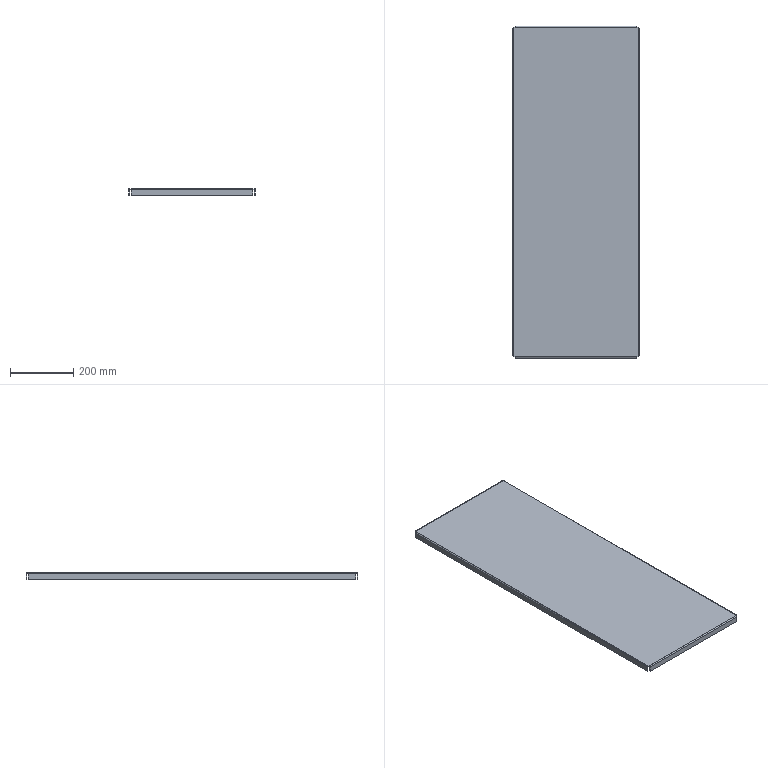Part | SolidWorks | features BaseBody 1 | 1 solid | 50 faces | box 398 x 1046 x 20 mm | volume 1158388 mm3 | plane 42 | cylinder 8 | commonest cylinder face diameters 1.473 x4 6.473 x4
STEP:
#1=CARTESIAN_POINT('',(-192.,-520.5,-20.));
#2=VERTEX_POINT('',#1);
#3=CARTESIAN_POINT('',(192.,-520.5,-20.));
#4=VERTEX_POINT('',#3);
#5=CARTESIAN_POINT('',(192.,-520.5,-20.));
#6=DIRECTION('',(1.,0.,0.));
#7=VECTOR('',#6,1000.);
#8=LINE('',#5,#7);
#9=EDGE_CURVE('',#2,#4,#8,.T.);
#10=ORIENTED_EDGE('',*,*,#9,.T.);
#11=CARTESIAN_POINT('',(192.,-523.,-20.));
#12=VERTEX_POINT('',#11);
#13=CARTESIAN_POINT('',(192.,-523.,-20.));
#14=DIRECTION('',(0.,1.,0.));
#15=VECTOR('',#14,1000.);
#16=LINE('',#13,#15);
#17=EDGE_CURVE('',#12,#4,#16,.T.);
#18=ORIENTED_EDGE('',*,*,#17,.F.);
#19=CARTESIAN_POINT('',(-192.,-523.,-20.));
#20=VERTEX_POINT('',#19);
#21=CARTESIAN_POINT('',(0.,-523.,-20.));
#22=DIRECTION('',(1.,0.,0.));
#23=VECTOR('',#22,1000.);
#24=LINE('',#21,#23);
#25=EDGE_CURVE('',#20,#12,#24,.T.);
#26=ORIENTED_EDGE('',*,*,#25,.F.);
#27=CARTESIAN_POINT('',(-192.,-523.,-20.));
#28=DIRECTION('',(0.,1.,0.));
#29=VECTOR('',#28,1000.);
#30=LINE('',#27,#29);
#31=EDGE_CURVE('',#20,#2,#30,.T.);
#32=ORIENTED_EDGE('',*,*,#31,.T.);
#33=EDGE_LOOP('',(#10,#18,#26,#32));
#34=FACE_OUTER_BOUND('',#33,.T.);
#35=CARTESIAN_POINT('',(192.,-523.,-20.));
#36=DIRECTION('',(0.,0.,1.));
#37=DIRECTION('',(0.,-1.,0.));
#38=AXIS2_PLACEMENT_3D('',#35,#36,#37);
#39=PLANE('',#38);
#40=ADVANCED_FACE('',(#34),#39,.F.);
#41=CARTESIAN_POINT('',(-192.,-520.5,-3.237));
#42=VERTEX_POINT('',#41);
#43=CARTESIAN_POINT('',(-192.,-520.5,-20.));
#44=DIRECTION('',(0.,0.,-1.));
#45=VECTOR('',#44,1000.);
#46=LINE('',#43,#45);
#47=EDGE_CURVE('',#42,#2,#46,.T.);
#48=ORIENTED_EDGE('',*,*,#47,.F.);
#49=CARTESIAN_POINT('',(192.,-520.5,-3.237));
#50=VERTEX_POINT('',#49);
#51=CARTESIAN_POINT('',(192.,-520.5,-3.237));
#52=DIRECTION('',(-1.,0.,0.));
#53=VECTOR('',#52,1000.);
#54=LINE('',#51,#53);
#55=EDGE_CURVE('',#50,#42,#54,.T.);
#56=ORIENTED_EDGE('',*,*,#55,.F.);
#57=CARTESIAN_POINT('',(192.,-520.5,-2.5));
#58=DIRECTION('',(0.,0.,1.));
#59=VECTOR('',#58,1000.);
#60=LINE('',#57,#59);
#61=EDGE_CURVE('',#4,#50,#60,.T.);
#62=ORIENTED_EDGE('',*,*,#61,.F.);
#63=ORIENTED_EDGE('',*,*,#9,.F.);
#64=EDGE_LOOP('',(#48,#56,#62,#63));
#65=FACE_OUTER_BOUND('',#64,.T.);
#66=CARTESIAN_POINT('',(0.,-520.5,0.));
#67=DIRECTION('',(0.,1.,0.));
#68=DIRECTION('',(1.,0.,0.));
#69=AXIS2_PLACEMENT_3D('',#66,#67,#68);
#70=PLANE('',#69);
#71=ADVANCED_FACE('',(#65),#70,.T.);
#72=CARTESIAN_POINT('',(-192.,-523.,-3.237));
#73=VERTEX_POINT('',#72);
#74=CARTESIAN_POINT('',(192.,-523.,-3.237));
#75=VERTEX_POINT('',#74);
#76=CARTESIAN_POINT('',(192.,-523.,-3.237));
#77=DIRECTION('',(1.,0.,0.));
#78=VECTOR('',#77,1000.);
#79=LINE('',#76,#78);
#80=EDGE_CURVE('',#73,#75,#79,.T.);
#81=ORIENTED_EDGE('',*,*,#80,.F.);
#82=CARTESIAN_POINT('',(-192.,-523.,0.));
#83=DIRECTION('',(0.,0.,-1.));
#84=VECTOR('',#83,1000.);
#85=LINE('',#82,#84);
#86=EDGE_CURVE('',#73,#20,#85,.T.);
#87=ORIENTED_EDGE('',*,*,#86,.T.);
#88=ORIENTED_EDGE('',*,*,#25,.T.);
#89=CARTESIAN_POINT('',(192.,-523.,0.));
#90=DIRECTION('',(0.,0.,1.));
#91=VECTOR('',#90,1000.);
#92=LINE('',#89,#91);
#93=EDGE_CURVE('',#12,#75,#92,.T.);
#94=ORIENTED_EDGE('',*,*,#93,.T.);
#95=EDGE_LOOP('',(#81,#87,#88,#94));
#96=FACE_OUTER_BOUND('',#95,.T.);
#97=CARTESIAN_POINT('',(0.,-523.,0.));
#98=DIRECTION('',(0.,1.,0.));
#99=DIRECTION('',(1.,0.,0.));
#100=AXIS2_PLACEMENT_3D('',#97,#98,#99);
#101=PLANE('',#100);
#102=ADVANCED_FACE('',(#96),#101,.F.);
#103=CARTESIAN_POINT('',(192.,-523.,-3.237));
#104=DIRECTION('',(0.,-1.,0.));
#105=VECTOR('',#104,1000.);
#106=LINE('',#103,#105);
#107=EDGE_CURVE('',#50,#75,#106,.T.);
#108=ORIENTED_EDGE('',*,*,#107,.T.);
#109=ORIENTED_EDGE('',*,*,#93,.F.);
#110=ORIENTED_EDGE('',*,*,#17,.T.);
#111=ORIENTED_EDGE('',*,*,#61,.T.);
#112=EDGE_LOOP('',(#108,#109,#110,#111));
#113=FACE_OUTER_BOUND('',#112,.T.);
#114=CARTESIAN_POINT('',(192.,-523.,-2.5));
#115=DIRECTION('',(-1.,0.,0.));
#116=DIRECTION('',(0.,1.,0.));
#117=AXIS2_PLACEMENT_3D('',#114,#115,#116);
#118=PLANE('',#117);
#119=ADVANCED_FACE('',(#113),#118,.F.);
#120=CARTESIAN_POINT('',(-192.,-520.5,-3.237));
#121=DIRECTION('',(0.,-1.,0.));
#122=VECTOR('',#121,1000.);
#123=LINE('',#120,#122);
#124=EDGE_CURVE('',#42,#73,#123,.T.);
#125=ORIENTED_EDGE('',*,*,#124,.F.);
#126=ORIENTED_EDGE('',*,*,#47,.T.);
#127=ORIENTED_EDGE('',*,*,#31,.F.);
#128=ORIENTED_EDGE('',*,*,#86,.F.);
#129=EDGE_LOOP('',(#125,#126,#127,#128));
#130=FACE_OUTER_BOUND('',#129,.T.);
#131=CARTESIAN_POINT('',(-192.,-523.,-20.));
#132=DIRECTION('',(1.,0.,0.));
#133=DIRECTION('',(0.,1.,0.));
#134=AXIS2_PLACEMENT_3D('',#131,#132,#133);
#135=PLANE('',#134);
#136=ADVANCED_FACE('',(#130),#135,.F.);
#137=CARTESIAN_POINT('',(-192.,-519.763,-2.5));
#138=VERTEX_POINT('',#137);
#139=CARTESIAN_POINT('',(192.,-519.763,-2.5));
#140=VERTEX_POINT('',#139);
#141=CARTESIAN_POINT('',(-192.,-519.763,-2.5));
#142=DIRECTION('',(1.,0.,0.));
#143=VECTOR('',#142,1000.);
#144=LINE('',#141,#143);
#145=EDGE_CURVE('',#138,#140,#144,.T.);
#146=ORIENTED_EDGE('',*,*,#145,.T.);
#147=CARTESIAN_POINT('',(192.,-519.763,-3.237));
#148=DIRECTION('',(1.,0.,0.));
#149=DIRECTION('',(0.,0.,1.));
#150=AXIS2_PLACEMENT_3D('',#147,#148,#149);
#151=CIRCLE('',#150,0.7366);
#152=EDGE_CURVE('',#140,#50,#151,.T.);
#153=ORIENTED_EDGE('',*,*,#152,.T.);
#154=ORIENTED_EDGE('',*,*,#55,.T.);
#155=CARTESIAN_POINT('',(-192.,-519.763,-3.237));
#156=DIRECTION('',(-1.,0.,0.));
#157=DIRECTION('',(0.,0.,1.));
#158=AXIS2_PLACEMENT_3D('',#155,#156,#157);
#159=CIRCLE('',#158,0.7366);
#160=EDGE_CURVE('',#42,#138,#159,.T.);
#161=ORIENTED_EDGE('',*,*,#160,.T.);
#162=EDGE_LOOP('',(#146,#153,#154,#161));
#163=FACE_OUTER_BOUND('',#162,.T.);
#164=CARTESIAN_POINT('',(-192.,-519.763,-3.237));
#165=DIRECTION('',(-1.,0.,0.));
#166=DIRECTION('',(0.,-1.,0.));
#167=AXIS2_PLACEMENT_3D('',#164,#165,#166);
#168=CYLINDRICAL_SURFACE('',#167,0.7366);
#169=ADVANCED_FACE('',(#163),#168,.F.);
#170=CARTESIAN_POINT('',(-192.,-519.763,0.));
#171=VERTEX_POINT('',#170);
#172=CARTESIAN_POINT('',(192.,-519.763,0.));
#173=VERTEX_POINT('',#172);
#174=CARTESIAN_POINT('',(-192.,-519.763,0.));
#175=DIRECTION('',(1.,0.,0.));
#176=VECTOR('',#175,1000.);
#177=LINE('',#174,#176);
#178=EDGE_CURVE('',#171,#173,#177,.T.);
#179=ORIENTED_EDGE('',*,*,#178,.F.);
#180=CARTESIAN_POINT('',(-192.,-522.915,-2.5));
#181=VERTEX_POINT('',#180);
#182=CARTESIAN_POINT('',(-192.,-519.763,-3.237));
#183=DIRECTION('',(-1.,0.,0.));
#184=DIRECTION('',(0.,0.,1.));
#185=AXIS2_PLACEMENT_3D('',#182,#183,#184);
#186=CIRCLE('',#185,3.237);
#187=EDGE_CURVE('',#181,#171,#186,.T.);
#188=ORIENTED_EDGE('',*,*,#187,.F.);
#189=CARTESIAN_POINT('',(-192.,-519.763,-3.237));
#190=DIRECTION('',(-1.,0.,0.));
#191=DIRECTION('',(0.,0.,1.));
#192=AXIS2_PLACEMENT_3D('',#189,#190,#191);
#193=CIRCLE('',#192,3.237);
#194=EDGE_CURVE('',#73,#181,#193,.T.);
#195=ORIENTED_EDGE('',*,*,#194,.F.);
#196=ORIENTED_EDGE('',*,*,#80,.T.);
#197=CARTESIAN_POINT('',(192.,-522.915,-2.5));
#198=VERTEX_POINT('',#197);
#199=CARTESIAN_POINT('',(192.,-519.763,-3.237));
#200=DIRECTION('',(1.,0.,0.));
#201=DIRECTION('',(0.,0.,1.));
#202=AXIS2_PLACEMENT_3D('',#199,#200,#201);
#203=CIRCLE('',#202,3.237);
#204=EDGE_CURVE('',#198,#75,#203,.T.);
#205=ORIENTED_EDGE('',*,*,#204,.F.);
#206=CARTESIAN_POINT('',(192.,-519.763,-3.237));
#207=DIRECTION('',(1.,0.,0.));
#208=DIRECTION('',(0.,0.,1.));
#209=AXIS2_PLACEMENT_3D('',#206,#207,#208);
#210=CIRCLE('',#209,3.237);
#211=EDGE_CURVE('',#173,#198,#210,.T.);
#212=ORIENTED_EDGE('',*,*,#211,.F.);
#213=EDGE_LOOP('',(#179,#188,#195,#196,#205,#212));
#214=FACE_OUTER_BOUND('',#213,.T.);
#215=CARTESIAN_POINT('',(-192.,-519.763,-3.237));
#216=DIRECTION('',(-1.,0.,0.));
#217=DIRECTION('',(0.,-1.,0.));
#218=AXIS2_PLACEMENT_3D('',#215,#216,#217);
#219=CYLINDRICAL_SURFACE('',#218,3.237);
#220=ADVANCED_FACE('',(#214),#219,.T.);
#221=ORIENTED_EDGE('',*,*,#194,.T.);
#222=CARTESIAN_POINT('',(-192.,-523.,-2.5));
#223=DIRECTION('',(0.,1.,0.));
#224=VECTOR('',#223,1000.);
#225=LINE('',#222,#224);
#226=EDGE_CURVE('',#181,#138,#225,.T.);
#227=ORIENTED_EDGE('',*,*,#226,.T.);
#228=ORIENTED_EDGE('',*,*,#160,.F.);
#229=ORIENTED_EDGE('',*,*,#124,.T.);
#230=EDGE_LOOP('',(#221,#227,#228,#229));
#231=FACE_OUTER_BOUND('',#230,.T.);
#232=CARTESIAN_POINT('',(-192.,-519.763,-3.237));
#233=DIRECTION('',(1.,0.,0.));
#234=DIRECTION('',(0.,1.,0.));
#235=AXIS2_PLACEMENT_3D('',#232,#233,#234);
#236=PLANE('',#235);
#237=ADVANCED_FACE('',(#231),#236,.F.);
#238=ORIENTED_EDGE('',*,*,#152,.F.);
#239=CARTESIAN_POINT('',(192.,-519.763,-2.5));
#240=DIRECTION('',(0.,-1.,0.));
#241=VECTOR('',#240,1000.);
#242=LINE('',#239,#241);
#243=EDGE_CURVE('',#140,#198,#242,.T.);
#244=ORIENTED_EDGE('',*,*,#243,.T.);
#245=ORIENTED_EDGE('',*,*,#204,.T.);
#246=ORIENTED_EDGE('',*,*,#107,.F.);
#247=EDGE_LOOP('',(#238,#244,#245,#246));
#248=FACE_OUTER_BOUND('',#247,.T.);
#249=CARTESIAN_POINT('',(192.,-519.763,-3.237));
#250=DIRECTION('',(1.,0.,0.));
#251=DIRECTION('',(0.,1.,0.));
#252=AXIS2_PLACEMENT_3D('',#249,#250,#251);
#253=PLANE('',#252);
#254=ADVANCED_FACE('',(#248),#253,.T.);
#255=CARTESIAN_POINT('',(196.5,-516.,-20.));
#256=VERTEX_POINT('',#255);
#257=CARTESIAN_POINT('',(196.5,516.,-20.));
#258=VERTEX_POINT('',#257);
#259=CARTESIAN_POINT('',(196.5,516.,-20.));
#260=DIRECTION('',(0.,1.,0.));
#261=VECTOR('',#260,1000.);
#262=LINE('',#259,#261);
#263=EDGE_CURVE('',#256,#258,#262,.T.);
#264=ORIENTED_EDGE('',*,*,#263,.T.);
#265=CARTESIAN_POINT('',(199.,516.,-20.));
#266=VERTEX_POINT('',#265);
#267=CARTESIAN_POINT('',(199.,516.,-20.));
#268=DIRECTION('',(-1.,0.,0.));
#269=VECTOR('',#268,1000.);
#270=LINE('',#267,#269);
#271=EDGE_CURVE('',#266,#258,#270,.T.);
#272=ORIENTED_EDGE('',*,*,#271,.F.);
#273=CARTESIAN_POINT('',(199.,-516.,-20.));
#274=VERTEX_POINT('',#273);
#275=CARTESIAN_POINT('',(199.,0.,-20.));
#276=DIRECTION('',(0.,1.,0.));
#277=VECTOR('',#276,1000.);
#278=LINE('',#275,#277);
#279=EDGE_CURVE('',#274,#266,#278,.T.);
#280=ORIENTED_EDGE('',*,*,#279,.F.);
#281=CARTESIAN_POINT('',(199.,-516.,-20.));
#282=DIRECTION('',(-1.,0.,0.));
#283=VECTOR('',#282,1000.);
#284=LINE('',#281,#283);
#285=EDGE_CURVE('',#274,#256,#284,.T.);
#286=ORIENTED_EDGE('',*,*,#285,.T.);
#287=EDGE_LOOP('',(#264,#272,#280,#286));
#288=FACE_OUTER_BOUND('',#287,.T.);
#289=CARTESIAN_POINT('',(199.,516.,-20.));
#290=DIRECTION('',(0.,0.,1.));
#291=DIRECTION('',(1.,0.,0.));
#292=AXIS2_PLACEMENT_3D('',#289,#290,#291);
#293=PLANE('',#292);
#294=ADVANCED_FACE('',(#288),#293,.F.);
#295=CARTESIAN_POINT('',(196.5,-516.,-3.237));
#296=VERTEX_POINT('',#295);
#297=CARTESIAN_POINT('',(196.5,-516.,-20.));
#298=DIRECTION('',(0.,0.,-1.));
#299=VECTOR('',#298,1000.);
#300=LINE('',#297,#299);
#301=EDGE_CURVE('',#296,#256,#300,.T.);
#302=ORIENTED_EDGE('',*,*,#301,.F.);
#303=CARTESIAN_POINT('',(196.5,516.,-3.237));
#304=VERTEX_POINT('',#303);
#305=CARTESIAN_POINT('',(196.5,516.,-3.237));
#306=DIRECTION('',(0.,-1.,0.));
#307=VECTOR('',#306,1000.);
#308=LINE('',#305,#307);
#309=EDGE_CURVE('',#304,#296,#308,.T.);
#310=ORIENTED_EDGE('',*,*,#309,.F.);
#311=CARTESIAN_POINT('',(196.5,516.,-2.5));
#312=DIRECTION('',(0.,0.,1.));
#313=VECTOR('',#312,1000.);
#314=LINE('',#311,#313);
#315=EDGE_CURVE('',#258,#304,#314,.T.);
#316=ORIENTED_EDGE('',*,*,#315,.F.);
#317=ORIENTED_EDGE('',*,*,#263,.F.);
#318=EDGE_LOOP('',(#302,#310,#316,#317));
#319=FACE_OUTER_BOUND('',#318,.T.);
#320=CARTESIAN_POINT('',(196.5,0.,0.));
#321=DIRECTION('',(-1.,0.,0.));
#322=DIRECTION('',(0.,0.,1.));
#323=AXIS2_PLACEMENT_3D('',#320,#321,#322);
#324=PLANE('',#323);
#325=ADVANCED_FACE('',(#319),#324,.T.);
#326=CARTESIAN_POINT('',(199.,-516.,-3.237));
#327=VERTEX_POINT('',#326);
#328=CARTESIAN_POINT('',(199.,516.,-3.237));
#329=VERTEX_POINT('',#328);
#330=CARTESIAN_POINT('',(199.,516.,-3.237));
#331=DIRECTION('',(0.,1.,0.));
#332=VECTOR('',#331,1000.);
#333=LINE('',#330,#332);
#334=EDGE_CURVE('',#327,#329,#333,.T.);
#335=ORIENTED_EDGE('',*,*,#334,.F.);
#336=CARTESIAN_POINT('',(199.,-516.,0.));
#337=DIRECTION('',(0.,0.,-1.));
#338=VECTOR('',#337,1000.);
#339=LINE('',#336,#338);
#340=EDGE_CURVE('',#327,#274,#339,.T.);
#341=ORIENTED_EDGE('',*,*,#340,.T.);
#342=ORIENTED_EDGE('',*,*,#279,.T.);
#343=CARTESIAN_POINT('',(199.,516.,0.));
#344=DIRECTION('',(0.,0.,1.));
#345=VECTOR('',#344,1000.);
#346=LINE('',#343,#345);
#347=EDGE_CURVE('',#266,#329,#346,.T.);
#348=ORIENTED_EDGE('',*,*,#347,.T.);
#349=EDGE_LOOP('',(#335,#341,#342,#348));
#350=FACE_OUTER_BOUND('',#349,.T.);
#351=CARTESIAN_POINT('',(199.,0.,0.));
#352=DIRECTION('',(-1.,0.,0.));
#353=DIRECTION('',(0.,0.,1.));
#354=AXIS2_PLACEMENT_3D('',#351,#352,#353);
#355=PLANE('',#354);
#356=ADVANCED_FACE('',(#350),#355,.F.);
#357=CARTESIAN_POINT('',(199.,516.,-3.237));
#358=DIRECTION('',(1.,0.,0.));
#359=VECTOR('',#358,1000.);
#360=LINE('',#357,#359);
#361=EDGE_CURVE('',#304,#329,#360,.T.);
#362=ORIENTED_EDGE('',*,*,#361,.T.);
#363=ORIENTED_EDGE('',*,*,#347,.F.);
#364=ORIENTED_EDGE('',*,*,#271,.T.);
#365=ORIENTED_EDGE('',*,*,#315,.T.);
#366=EDGE_LOOP('',(#362,#363,#364,#365));
#367=FACE_OUTER_BOUND('',#366,.T.);
#368=CARTESIAN_POINT('',(199.,516.,-2.5));
#369=DIRECTION('',(0.,-1.,0.));
#370=DIRECTION('',(0.,0.,-1.));
#371=AXIS2_PLACEMENT_3D('',#368,#369,#370);
#372=PLANE('',#371);
#373=ADVANCED_FACE('',(#367),#372,.F.);
#374=CARTESIAN_POINT('',(196.5,-516.,-3.237));
#375=DIRECTION('',(1.,0.,0.));
#376=VECTOR('',#375,1000.);
#377=LINE('',#374,#376);
#378=EDGE_CURVE('',#296,#327,#377,.T.);
#379=ORIENTED_EDGE('',*,*,#378,.F.);
#380=ORIENTED_EDGE('',*,*,#301,.T.);
#381=ORIENTED_EDGE('',*,*,#285,.F.);
#382=ORIENTED_EDGE('',*,*,#340,.F.);
#383=EDGE_LOOP('',(#379,#380,#381,#382));
#384=FACE_OUTER_BOUND('',#383,.T.);
#385=CARTESIAN_POINT('',(199.,-516.,-20.));
#386=DIRECTION('',(0.,1.,0.));
#387=DIRECTION('',(0.,0.,-1.));
#388=AXIS2_PLACEMENT_3D('',#385,#386,#387);
#389=PLANE('',#388);
#390=ADVANCED_FACE('',(#384),#389,.F.);
#391=CARTESIAN_POINT('',(195.763,-516.,-2.5));
#392=VERTEX_POINT('',#391);
#393=CARTESIAN_POINT('',(195.763,516.,-2.5));
#394=VERTEX_POINT('',#393);
#395=CARTESIAN_POINT('',(195.763,-516.,-2.5));
#396=DIRECTION('',(0.,1.,0.));
#397=VECTOR('',#396,1000.);
#398=LINE('',#395,#397);
#399=EDGE_CURVE('',#392,#394,#398,.T.);
#400=ORIENTED_EDGE('',*,*,#399,.T.);
#401=CARTESIAN_POINT('',(195.763,516.,-3.237));
#402=DIRECTION('',(0.,1.,0.));
#403=DIRECTION('',(0.,0.,-1.));
#404=AXIS2_PLACEMENT_3D('',#401,#402,#403);
#405=CIRCLE('',#404,0.7366);
#406=EDGE_CURVE('',#394,#304,#405,.T.);
#407=ORIENTED_EDGE('',*,*,#406,.T.);
#408=ORIENTED_EDGE('',*,*,#309,.T.);
#409=CARTESIAN_POINT('',(195.763,-516.,-3.237));
#410=DIRECTION('',(0.,-1.,0.));
#411=DIRECTION('',(0.,0.,-1.));
#412=AXIS2_PLACEMENT_3D('',#409,#410,#411);
#413=CIRCLE('',#412,0.7366);
#414=EDGE_CURVE('',#296,#392,#413,.T.);
#415=ORIENTED_EDGE('',*,*,#414,.T.);
#416=EDGE_LOOP('',(#400,#407,#408,#415));
#417=FACE_OUTER_BOUND('',#416,.T.);
#418=CARTESIAN_POINT('',(195.763,-516.,-3.237));
#419=DIRECTION('',(0.,-1.,0.));
#420=DIRECTION('',(1.,0.,0.));
#421=AXIS2_PLACEMENT_3D('',#418,#419,#420);
#422=CYLINDRICAL_SURFACE('',#421,0.7366);
#423=ADVANCED_FACE('',(#417),#422,.F.);
#424=CARTESIAN_POINT('',(195.763,-516.,0.));
#425=VERTEX_POINT('',#424);
#426=CARTESIAN_POINT('',(195.763,516.,0.));
#427=VERTEX_POINT('',#426);
#428=CARTESIAN_POINT('',(195.763,-516.,0.));
#429=DIRECTION('',(0.,1.,0.));
#430=VECTOR('',#429,1000.);
#431=LINE('',#428,#430);
#432=EDGE_CURVE('',#425,#427,#431,.T.);
#433=ORIENTED_EDGE('',*,*,#432,.F.);
#434=CARTESIAN_POINT('',(198.915,-516.,-2.5));
#435=VERTEX_POINT('',#434);
#436=CARTESIAN_POINT('',(195.763,-516.,-3.237));
#437=DIRECTION('',(0.,-1.,0.));
#438=DIRECTION('',(0.,0.,-1.));
#439=AXIS2_PLACEMENT_3D('',#436,#437,#438);
#440=CIRCLE('',#439,3.237);
#441=EDGE_CURVE('',#435,#425,#440,.T.);
#442=ORIENTED_EDGE('',*,*,#441,.F.);
#443=CARTESIAN_POINT('',(195.763,-516.,-3.237));
#444=DIRECTION('',(0.,-1.,0.));
#445=DIRECTION('',(0.,0.,-1.));
#446=AXIS2_PLACEMENT_3D('',#443,#444,#445);
#447=CIRCLE('',#446,3.237);
#448=EDGE_CURVE('',#327,#435,#447,.T.);
#449=ORIENTED_EDGE('',*,*,#448,.F.);
#450=ORIENTED_EDGE('',*,*,#334,.T.);
#451=CARTESIAN_POINT('',(198.915,516.,-2.5));
#452=VERTEX_POINT('',#451);
#453=CARTESIAN_POINT('',(195.763,516.,-3.237));
#454=DIRECTION('',(0.,1.,0.));
#455=DIRECTION('',(0.,0.,-1.));
#456=AXIS2_PLACEMENT_3D('',#453,#454,#455);
#457=CIRCLE('',#456,3.237);
#458=EDGE_CURVE('',#452,#329,#457,.T.);
#459=ORIENTED_EDGE('',*,*,#458,.F.);
#460=CARTESIAN_POINT('',(195.763,516.,-3.237));
#461=DIRECTION('',(0.,1.,0.));
#462=DIRECTION('',(0.,0.,-1.));
#463=AXIS2_PLACEMENT_3D('',#460,#461,#462);
#464=CIRCLE('',#463,3.237);
#465=EDGE_CURVE('',#427,#452,#464,.T.);
#466=ORIENTED_EDGE('',*,*,#465,.F.);
#467=EDGE_LOOP('',(#433,#442,#449,#450,#459,#466));
#468=FACE_OUTER_BOUND('',#467,.T.);
#469=CARTESIAN_POINT('',(195.763,-516.,-3.237));
#470=DIRECTION('',(0.,-1.,0.));
#471=DIRECTION('',(1.,0.,0.));
#472=AXIS2_PLACEMENT_3D('',#469,#470,#471);
#473=CYLINDRICAL_SURFACE('',#472,3.237);
#474=ADVANCED_FACE('',(#468),#473,.T.);
#475=ORIENTED_EDGE('',*,*,#448,.T.);
#476=CARTESIAN_POINT('',(199.,-516.,-2.5));
#477=DIRECTION('',(-1.,0.,0.));
#478=VECTOR('',#477,1000.);
#479=LINE('',#476,#478);
#480=EDGE_CURVE('',#435,#392,#479,.T.);
#481=ORIENTED_EDGE('',*,*,#480,.T.);
#482=ORIENTED_EDGE('',*,*,#414,.F.);
#483=ORIENTED_EDGE('',*,*,#378,.T.);
#484=EDGE_LOOP('',(#475,#481,#482,#483));
#485=FACE_OUTER_BOUND('',#484,.T.);
#486=CARTESIAN_POINT('',(195.763,-516.,-3.237));
#487=DIRECTION('',(0.,1.,0.));
#488=DIRECTION('',(0.,0.,-1.));
#489=AXIS2_PLACEMENT_3D('',#486,#487,#488);
#490=PLANE('',#489);
#491=ADVANCED_FACE('',(#485),#490,.F.);
#492=ORIENTED_EDGE('',*,*,#406,.F.);
#493=CARTESIAN_POINT('',(195.763,516.,-2.5));
#494=DIRECTION('',(1.,0.,0.));
#495=VECTOR('',#494,1000.);
#496=LINE('',#493,#495);
#497=EDGE_CURVE('',#394,#452,#496,.T.);
#498=ORIENTED_EDGE('',*,*,#497,.T.);
#499=ORIENTED_EDGE('',*,*,#458,.T.);
#500=ORIENTED_EDGE('',*,*,#361,.F.);
#501=EDGE_LOOP('',(#492,#498,#499,#500));
#502=FACE_OUTER_BOUND('',#501,.T.);
#503=CARTESIAN_POINT('',(195.763,516.,-3.237));
#504=DIRECTION('',(0.,1.,0.));
#505=DIRECTION('',(0.,0.,-1.));
#506=AXIS2_PLACEMENT_3D('',#503,#504,#505);
#507=PLANE('',#506);
#508=ADVANCED_FACE('',(#502),#507,.T.);
#509=CARTESIAN_POINT('',(192.,520.5,-20.));
#510=VERTEX_POINT('',#509);
#511=CARTESIAN_POINT('',(-192.,520.5,-20.));
#512=VERTEX_POINT('',#511);
#513=CARTESIAN_POINT('',(-192.,520.5,-20.));
#514=DIRECTION('',(-1.,0.,0.));
#515=VECTOR('',#514,1000.);
#516=LINE('',#513,#515);
#517=EDGE_CURVE('',#510,#512,#516,.T.);
#518=ORIENTED_EDGE('',*,*,#517,.T.);
#519=CARTESIAN_POINT('',(-192.,523.,-20.));
#520=VERTEX_POINT('',#519);
#521=CARTESIAN_POINT('',(-192.,523.,-20.));
#522=DIRECTION('',(0.,-1.,0.));
#523=VECTOR('',#522,1000.);
#524=LINE('',#521,#523);
#525=EDGE_CURVE('',#520,#512,#524,.T.);
#526=ORIENTED_EDGE('',*,*,#525,.F.);
#527=CARTESIAN_POINT('',(192.,523.,-20.));
#528=VERTEX_POINT('',#527);
#529=CARTESIAN_POINT('',(0.,523.,-20.));
#530=DIRECTION('',(-1.,0.,0.));
#531=VECTOR('',#530,1000.);
#532=LINE('',#529,#531);
#533=EDGE_CURVE('',#528,#520,#532,.T.);
#534=ORIENTED_EDGE('',*,*,#533,.F.);
#535=CARTESIAN_POINT('',(192.,523.,-20.));
#536=DIRECTION('',(0.,-1.,0.));
#537=VECTOR('',#536,1000.);
#538=LINE('',#535,#537);
#539=EDGE_CURVE('',#528,#510,#538,.T.);
#540=ORIENTED_EDGE('',*,*,#539,.T.);
#541=EDGE_LOOP('',(#518,#526,#534,#540));
#542=FACE_OUTER_BOUND('',#541,.T.);
#543=CARTESIAN_POINT('',(-192.,523.,-20.));
#544=DIRECTION('',(0.,0.,1.));
#545=DIRECTION('',(0.,-1.,0.));
#546=AXIS2_PLACEMENT_3D('',#543,#544,#545);
#547=PLANE('',#546);
#548=ADVANCED_FACE('',(#542),#547,.F.);
#549=CARTESIAN_POINT('',(192.,520.5,-3.237));
#550=VERTEX_POINT('',#549);
#551=CARTESIAN_POINT('',(192.,520.5,-20.));
#552=DIRECTION('',(0.,0.,-1.));
#553=VECTOR('',#552,1000.);
#554=LINE('',#551,#553);
#555=EDGE_CURVE('',#550,#510,#554,.T.);
#556=ORIENTED_EDGE('',*,*,#555,.F.);
#557=CARTESIAN_POINT('',(-192.,520.5,-3.237));
#558=VERTEX_POINT('',#557);
#559=CARTESIAN_POINT('',(-192.,520.5,-3.237));
#560=DIRECTION('',(1.,0.,0.));
#561=VECTOR('',#560,1000.);
#562=LINE('',#559,#561);
#563=EDGE_CURVE('',#558,#550,#562,.T.);
#564=ORIENTED_EDGE('',*,*,#563,.F.);
#565=CARTESIAN_POINT('',(-192.,520.5,-2.5));
#566=DIRECTION('',(0.,0.,1.));
#567=VECTOR('',#566,1000.);
#568=LINE('',#565,#567);
#569=EDGE_CURVE('',#512,#558,#568,.T.);
#570=ORIENTED_EDGE('',*,*,#569,.F.);
#571=ORIENTED_EDGE('',*,*,#517,.F.);
#572=EDGE_LOOP('',(#556,#564,#570,#571));
#573=FACE_OUTER_BOUND('',#572,.T.);
#574=CARTESIAN_POINT('',(0.,520.5,0.));
#575=DIRECTION('',(0.,-1.,0.));
#576=DIRECTION('',(-1.,0.,0.));
#577=AXIS2_PLACEMENT_3D('',#574,#575,#576);
#578=PLANE('',#577);
#579=ADVANCED_FACE('',(#573),#578,.T.);
#580=CARTESIAN_POINT('',(192.,523.,-3.237));
#581=VERTEX_POINT('',#580);
#582=CARTESIAN_POINT('',(-192.,523.,-3.237));
#583=VERTEX_POINT('',#582);
#584=CARTESIAN_POINT('',(-192.,523.,-3.237));
#585=DIRECTION('',(-1.,0.,0.));
#586=VECTOR('',#585,1000.);
#587=LINE('',#584,#586);
#588=EDGE_CURVE('',#581,#583,#587,.T.);
#589=ORIENTED_EDGE('',*,*,#588,.F.);
#590=CARTESIAN_POINT('',(192.,523.,0.));
#591=DIRECTION('',(0.,0.,-1.));
#592=VECTOR('',#591,1000.);
#593=LINE('',#590,#592);
#594=EDGE_CURVE('',#581,#528,#593,.T.);
#595=ORIENTED_EDGE('',*,*,#594,.T.);
#596=ORIENTED_EDGE('',*,*,#533,.T.);
#597=CARTESIAN_POINT('',(-192.,523.,0.));
#598=DIRECTION('',(0.,0.,1.));
#599=VECTOR('',#598,1000.);
#600=LINE('',#597,#599);
#601=EDGE_CURVE('',#520,#583,#600,.T.);
#602=ORIENTED_EDGE('',*,*,#601,.T.);
#603=EDGE_LOOP('',(#589,#595,#596,#602));
#604=FACE_OUTER_BOUND('',#603,.T.);
#605=CARTESIAN_POINT('',(0.,523.,0.));
#606=DIRECTION('',(0.,-1.,0.));
#607=DIRECTION('',(-1.,0.,0.));
#608=AXIS2_PLACEMENT_3D('',#605,#606,#607);
#609=PLANE('',#608);
#610=ADVANCED_FACE('',(#604),#609,.F.);
#611=CARTESIAN_POINT('',(-192.,523.,-3.237));
#612=DIRECTION('',(0.,1.,0.));
#613=VECTOR('',#612,1000.);
#614=LINE('',#611,#613);
#615=EDGE_CURVE('',#558,#583,#614,.T.);
#616=ORIENTED_EDGE('',*,*,#615,.T.);
#617=ORIENTED_EDGE('',*,*,#601,.F.);
#618=ORIENTED_EDGE('',*,*,#525,.T.);
#619=ORIENTED_EDGE('',*,*,#569,.T.);
#620=EDGE_LOOP('',(#616,#617,#618,#619));
#621=FACE_OUTER_BOUND('',#620,.T.);
#622=CARTESIAN_POINT('',(-192.,523.,-2.5));
#623=DIRECTION('',(1.,0.,0.));
#624=DIRECTION('',(0.,-1.,0.));
#625=AXIS2_PLACEMENT_3D('',#622,#623,#624);
#626=PLANE('',#625);
#627=ADVANCED_FACE('',(#621),#626,.F.);
#628=CARTESIAN_POINT('',(192.,520.5,-3.237));
#629=DIRECTION('',(0.,1.,0.));
#630=VECTOR('',#629,1000.);
#631=LINE('',#628,#630);
#632=EDGE_CURVE('',#550,#581,#631,.T.);
#633=ORIENTED_EDGE('',*,*,#632,.F.);
#634=ORIENTED_EDGE('',*,*,#555,.T.);
#635=ORIENTED_EDGE('',*,*,#539,.F.);
#636=ORIENTED_EDGE('',*,*,#594,.F.);
#637=EDGE_LOOP('',(#633,#634,#635,#636));
#638=FACE_OUTER_BOUND('',#637,.T.);
#639=CARTESIAN_POINT('',(192.,523.,-20.));
#640=DIRECTION('',(-1.,0.,0.));
#641=DIRECTION('',(0.,0.,1.));
#642=AXIS2_PLACEMENT_3D('',#639,#640,#641);
#643=PLANE('',#642);
#644=ADVANCED_FACE('',(#638),#643,.F.);
#645=CARTESIAN_POINT('',(192.,519.763,-2.5));
#646=VERTEX_POINT('',#645);
#647=CARTESIAN_POINT('',(-192.,519.763,-2.5));
#648=VERTEX_POINT('',#647);
#649=CARTESIAN_POINT('',(192.,519.763,-2.5));
#650=DIRECTION('',(-1.,0.,0.));
#651=VECTOR('',#650,1000.);
#652=LINE('',#649,#651);
#653=EDGE_CURVE('',#646,#648,#652,.T.);
#654=ORIENTED_EDGE('',*,*,#653,.T.);
#655=CARTESIAN_POINT('',(-192.,519.763,-3.237));
#656=DIRECTION('',(-1.,0.,0.));
#657=DIRECTION('',(0.,0.,-1.));
#658=AXIS2_PLACEMENT_3D('',#655,#656,#657);
#659=CIRCLE('',#658,0.7366);
#660=EDGE_CURVE('',#648,#558,#659,.T.);
#661=ORIENTED_EDGE('',*,*,#660,.T.);
#662=ORIENTED_EDGE('',*,*,#563,.T.);
#663=CARTESIAN_POINT('',(192.,519.763,-3.237));
#664=DIRECTION('',(1.,0.,0.));
#665=DIRECTION('',(0.,0.,-1.));
#666=AXIS2_PLACEMENT_3D('',#663,#664,#665);
#667=CIRCLE('',#666,0.7366);
#668=EDGE_CURVE('',#550,#646,#667,.T.);
#669=ORIENTED_EDGE('',*,*,#668,.T.);
#670=EDGE_LOOP('',(#654,#661,#662,#669));
#671=FACE_OUTER_BOUND('',#670,.T.);
#672=CARTESIAN_POINT('',(192.,519.763,-3.237));
#673=DIRECTION('',(1.,0.,0.));
#674=DIRECTION('',(0.,1.,0.));
#675=AXIS2_PLACEMENT_3D('',#672,#673,#674);
#676=CYLINDRICAL_SURFACE('',#675,0.7366);
#677=ADVANCED_FACE('',(#671),#676,.F.);
#678=CARTESIAN_POINT('',(192.,519.763,0.));
#679=VERTEX_POINT('',#678);
#680=CARTESIAN_POINT('',(-192.,519.763,0.));
#681=VERTEX_POINT('',#680);
#682=CARTESIAN_POINT('',(192.,519.763,0.));
#683=DIRECTION('',(-1.,0.,0.));
#684=VECTOR('',#683,1000.);
#685=LINE('',#682,#684);
#686=EDGE_CURVE('',#679,#681,#685,.T.);
#687=ORIENTED_EDGE('',*,*,#686,.F.);
#688=CARTESIAN_POINT('',(192.,522.915,-2.5));
#689=VERTEX_POINT('',#688);
#690=CARTESIAN_POINT('',(192.,519.763,-3.237));
#691=DIRECTION('',(1.,0.,0.));
#692=DIRECTION('',(0.,0.,-1.));
#693=AXIS2_PLACEMENT_3D('',#690,#691,#692);
#694=CIRCLE('',#693,3.237);
#695=EDGE_CURVE('',#689,#679,#694,.T.);
#696=ORIENTED_EDGE('',*,*,#695,.F.);
#697=CARTESIAN_POINT('',(192.,519.763,-3.237));
#698=DIRECTION('',(1.,0.,0.));
#699=DIRECTION('',(0.,0.,-1.));
#700=AXIS2_PLACEMENT_3D('',#697,#698,#699);
#701=CIRCLE('',#700,3.237);
#702=EDGE_CURVE('',#581,#689,#701,.T.);
#703=ORIENTED_EDGE('',*,*,#702,.F.);
#704=ORIENTED_EDGE('',*,*,#588,.T.);
#705=CARTESIAN_POINT('',(-192.,522.915,-2.5));
#706=VERTEX_POINT('',#705);
#707=CARTESIAN_POINT('',(-192.,519.763,-3.237));
#708=DIRECTION('',(-1.,0.,0.));
#709=DIRECTION('',(0.,0.,-1.));
#710=AXIS2_PLACEMENT_3D('',#707,#708,#709);
#711=CIRCLE('',#710,3.237);
#712=EDGE_CURVE('',#706,#583,#711,.T.);
#713=ORIENTED_EDGE('',*,*,#712,.F.);
#714=CARTESIAN_POINT('',(-192.,519.763,-3.237));
#715=DIRECTION('',(-1.,0.,0.));
#716=DIRECTION('',(0.,0.,-1.));
#717=AXIS2_PLACEMENT_3D('',#714,#715,#716);
#718=CIRCLE('',#717,3.237);
#719=EDGE_CURVE('',#681,#706,#718,.T.);
#720=ORIENTED_EDGE('',*,*,#719,.F.);
#721=EDGE_LOOP('',(#687,#696,#703,#704,#713,#720));
#722=FACE_OUTER_BOUND('',#721,.T.);
#723=CARTESIAN_POINT('',(192.,519.763,-3.237));
#724=DIRECTION('',(1.,0.,0.));
#725=DIRECTION('',(0.,1.,0.));
#726=AXIS2_PLACEMENT_3D('',#723,#724,#725);
#727=CYLINDRICAL_SURFACE('',#726,3.237);
#728=ADVANCED_FACE('',(#722),#727,.T.);
#729=ORIENTED_EDGE('',*,*,#702,.T.);
#730=CARTESIAN_POINT('',(192.,523.,-2.5));
#731=DIRECTION('',(0.,-1.,0.));
#732=VECTOR('',#731,1000.);
#733=LINE('',#730,#732);
#734=EDGE_CURVE('',#689,#646,#733,.T.);
#735=ORIENTED_EDGE('',*,*,#734,.T.);
#736=ORIENTED_EDGE('',*,*,#668,.F.);
#737=ORIENTED_EDGE('',*,*,#632,.T.);
#738=EDGE_LOOP('',(#729,#735,#736,#737));
#739=FACE_OUTER_BOUND('',#738,.T.);
#740=CARTESIAN_POINT('',(192.,519.763,-3.237));
#741=DIRECTION('',(-1.,0.,0.));
#742=DIRECTION('',(0.,0.,1.));
#743=AXIS2_PLACEMENT_3D('',#740,#741,#742);
#744=PLANE('',#743);
#745=ADVANCED_FACE('',(#739),#744,.F.);
#746=ORIENTED_EDGE('',*,*,#660,.F.);
#747=CARTESIAN_POINT('',(-192.,519.763,-2.5));
#748=DIRECTION('',(0.,1.,0.));
#749=VECTOR('',#748,1000.);
#750=LINE('',#747,#749);
#751=EDGE_CURVE('',#648,#706,#750,.T.);
#752=ORIENTED_EDGE('',*,*,#751,.T.);
#753=ORIENTED_EDGE('',*,*,#712,.T.);
#754=ORIENTED_EDGE('',*,*,#615,.F.);
#755=EDGE_LOOP('',(#746,#752,#753,#754));
#756=FACE_OUTER_BOUND('',#755,.T.);
#757=CARTESIAN_POINT('',(-192.,519.763,-3.237));
#758=DIRECTION('',(-1.,0.,0.));
#759=DIRECTION('',(0.,0.,1.));
#760=AXIS2_PLACEMENT_3D('',#757,#758,#759);
#761=PLANE('',#760);
#762=ADVANCED_FACE('',(#756),#761,.T.);
#763=CARTESIAN_POINT('',(-196.5,516.,-20.));
#764=VERTEX_POINT('',#763);
#765=CARTESIAN_POINT('',(-196.5,-516.,-20.));
#766=VERTEX_POINT('',#765);
#767=CARTESIAN_POINT('',(-196.5,-516.,-20.));
#768=DIRECTION('',(0.,-1.,0.));
#769=VECTOR('',#768,1000.);
#770=LINE('',#767,#769);
#771=EDGE_CURVE('',#764,#766,#770,.T.);
#772=ORIENTED_EDGE('',*,*,#771,.T.);
#773=CARTESIAN_POINT('',(-199.,-516.,-20.));
#774=VERTEX_POINT('',#773);
#775=CARTESIAN_POINT('',(-199.,-516.,-20.));
#776=DIRECTION('',(1.,0.,0.));
#777=VECTOR('',#776,1000.);
#778=LINE('',#775,#777);
#779=EDGE_CURVE('',#774,#766,#778,.T.);
#780=ORIENTED_EDGE('',*,*,#779,.F.);
#781=CARTESIAN_POINT('',(-199.,516.,-20.));
#782=VERTEX_POINT('',#781);
#783=CARTESIAN_POINT('',(-199.,0.,-20.));
#784=DIRECTION('',(0.,-1.,0.));
#785=VECTOR('',#784,1000.);
#786=LINE('',#783,#785);
#787=EDGE_CURVE('',#782,#774,#786,.T.);
#788=ORIENTED_EDGE('',*,*,#787,.F.);
#789=CARTESIAN_POINT('',(-199.,516.,-20.));
#790=DIRECTION('',(1.,0.,0.));
#791=VECTOR('',#790,1000.);
#792=LINE('',#789,#791);
#793=EDGE_CURVE('',#782,#764,#792,.T.);
#794=ORIENTED_EDGE('',*,*,#793,.T.);
#795=EDGE_LOOP('',(#772,#780,#788,#794));
#796=FACE_OUTER_BOUND('',#795,.T.);
#797=CARTESIAN_POINT('',(-199.,-516.,-20.));
#798=DIRECTION('',(0.,0.,1.));
#799=DIRECTION('',(1.,0.,0.));
#800=AXIS2_PLACEMENT_3D('',#797,#798,#799);
#801=PLANE('',#800);
#802=ADVANCED_FACE('',(#796),#801,.F.);
#803=CARTESIAN_POINT('',(-196.5,516.,-3.237));
#804=VERTEX_POINT('',#803);
#805=CARTESIAN_POINT('',(-196.5,516.,-20.));
#806=DIRECTION('',(0.,0.,-1.));
#807=VECTOR('',#806,1000.);
#808=LINE('',#805,#807);
#809=EDGE_CURVE('',#804,#764,#808,.T.);
#810=ORIENTED_EDGE('',*,*,#809,.F.);
#811=CARTESIAN_POINT('',(-196.5,-516.,-3.237));
#812=VERTEX_POINT('',#811);
#813=CARTESIAN_POINT('',(-196.5,-516.,-3.237));
#814=DIRECTION('',(0.,1.,0.));
#815=VECTOR('',#814,1000.);
#816=LINE('',#813,#815);
#817=EDGE_CURVE('',#812,#804,#816,.T.);
#818=ORIENTED_EDGE('',*,*,#817,.F.);
#819=CARTESIAN_POINT('',(-196.5,-516.,-2.5));
#820=DIRECTION('',(0.,0.,1.));
#821=VECTOR('',#820,1000.);
#822=LINE('',#819,#821);
#823=EDGE_CURVE('',#766,#812,#822,.T.);
#824=ORIENTED_EDGE('',*,*,#823,.F.);
#825=ORIENTED_EDGE('',*,*,#771,.F.);
#826=EDGE_LOOP('',(#810,#818,#824,#825));
#827=FACE_OUTER_BOUND('',#826,.T.);
#828=CARTESIAN_POINT('',(-196.5,0.,0.));
#829=DIRECTION('',(1.,0.,0.));
#830=DIRECTION('',(0.,0.,-1.));
#831=AXIS2_PLACEMENT_3D('',#828,#829,#830);
#832=PLANE('',#831);
#833=ADVANCED_FACE('',(#827),#832,.T.);
#834=CARTESIAN_POINT('',(-199.,516.,-3.237));
#835=VERTEX_POINT('',#834);
#836=CARTESIAN_POINT('',(-199.,-516.,-3.237));
#837=VERTEX_POINT('',#836);
#838=CARTESIAN_POINT('',(-199.,-516.,-3.237));
#839=DIRECTION('',(0.,-1.,0.));
#840=VECTOR('',#839,1000.);
#841=LINE('',#838,#840);
#842=EDGE_CURVE('',#835,#837,#841,.T.);
#843=ORIENTED_EDGE('',*,*,#842,.F.);
#844=CARTESIAN_POINT('',(-199.,516.,0.));
#845=DIRECTION('',(0.,0.,-1.));
#846=VECTOR('',#845,1000.);
#847=LINE('',#844,#846);
#848=EDGE_CURVE('',#835,#782,#847,.T.);
#849=ORIENTED_EDGE('',*,*,#848,.T.);
#850=ORIENTED_EDGE('',*,*,#787,.T.);
#851=CARTESIAN_POINT('',(-199.,-516.,0.));
#852=DIRECTION('',(0.,0.,1.));
#853=VECTOR('',#852,1000.);
#854=LINE('',#851,#853);
#855=EDGE_CURVE('',#774,#837,#854,.T.);
#856=ORIENTED_EDGE('',*,*,#855,.T.);
#857=EDGE_LOOP('',(#843,#849,#850,#856));
#858=FACE_OUTER_BOUND('',#857,.T.);
#859=CARTESIAN_POINT('',(-199.,0.,0.));
#860=DIRECTION('',(1.,0.,0.));
#861=DIRECTION('',(0.,0.,-1.));
#862=AXIS2_PLACEMENT_3D('',#859,#860,#861);
#863=PLANE('',#862);
#864=ADVANCED_FACE('',(#858),#863,.F.);
#865=CARTESIAN_POINT('',(-199.,-516.,-3.237));
#866=DIRECTION('',(-1.,0.,0.));
#867=VECTOR('',#866,1000.);
#868=LINE('',#865,#867);
#869=EDGE_CURVE('',#812,#837,#868,.T.);
#870=ORIENTED_EDGE('',*,*,#869,.T.);
#871=ORIENTED_EDGE('',*,*,#855,.F.);
#872=ORIENTED_EDGE('',*,*,#779,.T.);
#873=ORIENTED_EDGE('',*,*,#823,.T.);
#874=EDGE_LOOP('',(#870,#871,#872,#873));
#875=FACE_OUTER_BOUND('',#874,.T.);
#876=CARTESIAN_POINT('',(-199.,-516.,-2.5));
#877=DIRECTION('',(0.,1.,0.));
#878=DIRECTION('',(0.,0.,-1.));
#879=AXIS2_PLACEMENT_3D('',#876,#877,#878);
#880=PLANE('',#879);
#881=ADVANCED_FACE('',(#875),#880,.F.);
#882=CARTESIAN_POINT('',(-196.5,516.,-3.237));
#883=DIRECTION('',(-1.,0.,0.));
#884=VECTOR('',#883,1000.);
#885=LINE('',#882,#884);
#886=EDGE_CURVE('',#804,#835,#885,.T.);
#887=ORIENTED_EDGE('',*,*,#886,.F.);
#888=ORIENTED_EDGE('',*,*,#809,.T.);
#889=ORIENTED_EDGE('',*,*,#793,.F.);
#890=ORIENTED_EDGE('',*,*,#848,.F.);
#891=EDGE_LOOP('',(#887,#888,#889,#890));
#892=FACE_OUTER_BOUND('',#891,.T.);
#893=CARTESIAN_POINT('',(-199.,516.,-20.));
#894=DIRECTION('',(0.,-1.,0.));
#895=DIRECTION('',(-1.,0.,0.));
#896=AXIS2_PLACEMENT_3D('',#893,#894,#895);
#897=PLANE('',#896);
#898=ADVANCED_FACE('',(#892),#897,.F.);
#899=CARTESIAN_POINT('',(-195.763,516.,-2.5));
#900=VERTEX_POINT('',#899);
#901=CARTESIAN_POINT('',(-195.763,-516.,-2.5));
#902=VERTEX_POINT('',#901);
#903=CARTESIAN_POINT('',(-195.763,516.,-2.5));
#904=DIRECTION('',(0.,-1.,0.));
#905=VECTOR('',#904,1000.);
#906=LINE('',#903,#905);
#907=EDGE_CURVE('',#900,#902,#906,.T.);
#908=ORIENTED_EDGE('',*,*,#907,.T.);
#909=CARTESIAN_POINT('',(-195.763,-516.,-3.237));
#910=DIRECTION('',(0.,-1.,0.));
#911=DIRECTION('',(0.,0.,1.));
#912=AXIS2_PLACEMENT_3D('',#909,#910,#911);
#913=CIRCLE('',#912,0.7366);
#914=EDGE_CURVE('',#902,#812,#913,.T.);
#915=ORIENTED_EDGE('',*,*,#914,.T.);
#916=ORIENTED_EDGE('',*,*,#817,.T.);
#917=CARTESIAN_POINT('',(-195.763,516.,-3.237));
#918=DIRECTION('',(0.,1.,0.));
#919=DIRECTION('',(0.,0.,1.));
#920=AXIS2_PLACEMENT_3D('',#917,#918,#919);
#921=CIRCLE('',#920,0.7366);
#922=EDGE_CURVE('',#804,#900,#921,.T.);
#923=ORIENTED_EDGE('',*,*,#922,.T.);
#924=EDGE_LOOP('',(#908,#915,#916,#923));
#925=FACE_OUTER_BOUND('',#924,.T.);
#926=CARTESIAN_POINT('',(-195.763,516.,-3.237));
#927=DIRECTION('',(0.,1.,0.));
#928=DIRECTION('',(-1.,0.,0.));
#929=AXIS2_PLACEMENT_3D('',#926,#927,#928);
#930=CYLINDRICAL_SURFACE('',#929,0.7366);
#931=ADVANCED_FACE('',(#925),#930,.F.);
#932=CARTESIAN_POINT('',(-195.763,516.,0.));
#933=VERTEX_POINT('',#932);
#934=CARTESIAN_POINT('',(-195.763,-516.,0.));
#935=VERTEX_POINT('',#934);
#936=CARTESIAN_POINT('',(-195.763,516.,0.));
#937=DIRECTION('',(0.,-1.,0.));
#938=VECTOR('',#937,1000.);
#939=LINE('',#936,#938);
#940=EDGE_CURVE('',#933,#935,#939,.T.);
#941=ORIENTED_EDGE('',*,*,#940,.F.);
#942=CARTESIAN_POINT('',(-198.915,516.,-2.5));
#943=VERTEX_POINT('',#942);
#944=CARTESIAN_POINT('',(-195.763,516.,-3.237));
#945=DIRECTION('',(0.,1.,0.));
#946=DIRECTION('',(0.,0.,1.));
#947=AXIS2_PLACEMENT_3D('',#944,#945,#946);
#948=CIRCLE('',#947,3.237);
#949=EDGE_CURVE('',#943,#933,#948,.T.);
#950=ORIENTED_EDGE('',*,*,#949,.F.);
#951=CARTESIAN_POINT('',(-195.763,516.,-3.237));
#952=DIRECTION('',(0.,1.,0.));
#953=DIRECTION('',(0.,0.,1.));
#954=AXIS2_PLACEMENT_3D('',#951,#952,#953);
#955=CIRCLE('',#954,3.237);
#956=EDGE_CURVE('',#835,#943,#955,.T.);
#957=ORIENTED_EDGE('',*,*,#956,.F.);
#958=ORIENTED_EDGE('',*,*,#842,.T.);
#959=CARTESIAN_POINT('',(-198.915,-516.,-2.5));
#960=VERTEX_POINT('',#959);
#961=CARTESIAN_POINT('',(-195.763,-516.,-3.237));
#962=DIRECTION('',(0.,-1.,0.));
#963=DIRECTION('',(0.,0.,1.));
#964=AXIS2_PLACEMENT_3D('',#961,#962,#963);
#965=CIRCLE('',#964,3.237);
#966=EDGE_CURVE('',#960,#837,#965,.T.);
#967=ORIENTED_EDGE('',*,*,#966,.F.);
#968=CARTESIAN_POINT('',(-195.763,-516.,-3.237));
#969=DIRECTION('',(0.,-1.,0.));
#970=DIRECTION('',(0.,0.,1.));
#971=AXIS2_PLACEMENT_3D('',#968,#969,#970);
#972=CIRCLE('',#971,3.237);
#973=EDGE_CURVE('',#935,#960,#972,.T.);
#974=ORIENTED_EDGE('',*,*,#973,.F.);
#975=EDGE_LOOP('',(#941,#950,#957,#958,#967,#974));
#976=FACE_OUTER_BOUND('',#975,.T.);
#977=CARTESIAN_POINT('',(-195.763,516.,-3.237));
#978=DIRECTION('',(0.,1.,0.));
#979=DIRECTION('',(-1.,0.,0.));
#980=AXIS2_PLACEMENT_3D('',#977,#978,#979);
#981=CYLINDRICAL_SURFACE('',#980,3.237);
#982=ADVANCED_FACE('',(#976),#981,.T.);
#983=ORIENTED_EDGE('',*,*,#956,.T.);
#984=CARTESIAN_POINT('',(-199.,516.,-2.5));
#985=DIRECTION('',(1.,0.,0.));
#986=VECTOR('',#985,1000.);
#987=LINE('',#984,#986);
#988=EDGE_CURVE('',#943,#900,#987,.T.);
#989=ORIENTED_EDGE('',*,*,#988,.T.);
#990=ORIENTED_EDGE('',*,*,#922,.F.);
#991=ORIENTED_EDGE('',*,*,#886,.T.);
#992=EDGE_LOOP('',(#983,#989,#990,#991));
#993=FACE_OUTER_BOUND('',#992,.T.);
#994=CARTESIAN_POINT('',(-195.763,516.,-3.237));
#995=DIRECTION('',(0.,-1.,0.));
#996=DIRECTION('',(0.,0.,-1.));
#997=AXIS2_PLACEMENT_3D('',#994,#995,#996);
#998=PLANE('',#997);
#999=ADVANCED_FACE('',(#993),#998,.F.);
#1000=ORIENTED_EDGE('',*,*,#914,.F.);
#1001=CARTESIAN_POINT('',(-195.763,-516.,-2.5));
#1002=DIRECTION('',(-1.,0.,0.));
#1003=VECTOR('',#1002,1000.);
#1004=LINE('',#1001,#1003);
#1005=EDGE_CURVE('',#902,#960,#1004,.T.);
#1006=ORIENTED_EDGE('',*,*,#1005,.T.);
#1007=ORIENTED_EDGE('',*,*,#966,.T.);
#1008=ORIENTED_EDGE('',*,*,#869,.F.);
#1009=EDGE_LOOP('',(#1000,#1006,#1007,#1008));
#1010=FACE_OUTER_BOUND('',#1009,.T.);
#1011=CARTESIAN_POINT('',(-195.763,-516.,-3.237));
#1012=DIRECTION('',(0.,-1.,0.));
#1013=DIRECTION('',(0.,0.,-1.));
#1014=AXIS2_PLACEMENT_3D('',#1011,#1012,#1013);
#1015=PLANE('',#1014);
#1016=ADVANCED_FACE('',(#1010),#1015,.T.);
#1017=CARTESIAN_POINT('',(199.,-516.,-2.5));
#1018=VERTEX_POINT('',#1017);
#1019=CARTESIAN_POINT('',(192.,-523.,-2.5));
#1020=VERTEX_POINT('',#1019);
#1021=CARTESIAN_POINT('',(357.5,-357.5,-2.5));
#1022=DIRECTION('',(-0.7071,-0.7071,0.));
#1023=VECTOR('',#1022,1000.);
#1024=LINE('',#1021,#1023);
#1025=EDGE_CURVE('',#1018,#1020,#1024,.T.);
#1026=ORIENTED_EDGE('',*,*,#1025,.F.);
#1027=CARTESIAN_POINT('',(199.,-516.,0.));
#1028=VERTEX_POINT('',#1027);
#1029=CARTESIAN_POINT('',(199.,-516.,-2.5));
#1030=DIRECTION('',(0.,0.,-1.));
#1031=VECTOR('',#1030,1000.);
#1032=LINE('',#1029,#1031);
#1033=EDGE_CURVE('',#1028,#1018,#1032,.T.);
#1034=ORIENTED_EDGE('',*,*,#1033,.F.);
#1035=CARTESIAN_POINT('',(192.,-523.,0.));
#1036=VERTEX_POINT('',#1035);
#1037=CARTESIAN_POINT('',(192.,-523.,0.));
#1038=DIRECTION('',(0.7071,0.7071,0.));
#1039=VECTOR('',#1038,1000.);
#1040=LINE('',#1037,#1039);
#1041=EDGE_CURVE('',#1036,#1028,#1040,.T.);
#1042=ORIENTED_EDGE('',*,*,#1041,.F.);
#1043=CARTESIAN_POINT('',(192.,-523.,-2.5));
#1044=DIRECTION('',(0.,0.,1.));
#1045=VECTOR('',#1044,1000.);
#1046=LINE('',#1043,#1045);
#1047=EDGE_CURVE('',#1020,#1036,#1046,.T.);
#1048=ORIENTED_EDGE('',*,*,#1047,.F.);
#1049=EDGE_LOOP('',(#1026,#1034,#1042,#1048));
#1050=FACE_OUTER_BOUND('',#1049,.T.);
#1051=CARTESIAN_POINT('',(192.,-523.,-2.5));
#1052=DIRECTION('',(-0.7071,0.7071,0.));
#1053=DIRECTION('',(0.,0.,1.));
#1054=AXIS2_PLACEMENT_3D('',#1051,#1052,#1053);
#1055=PLANE('',#1054);
#1056=ADVANCED_FACE('',(#1050),#1055,.F.);
#1057=CARTESIAN_POINT('',(-192.,-523.,-2.5));
#1058=VERTEX_POINT('',#1057);
#1059=CARTESIAN_POINT('',(-199.,-516.,-2.5));
#1060=VERTEX_POINT('',#1059);
#1061=CARTESIAN_POINT('',(-357.5,-357.5,-2.5));
#1062=DIRECTION('',(-0.7071,0.7071,0.));
#1063=VECTOR('',#1062,1000.);
#1064=LINE('',#1061,#1063);
#1065=EDGE_CURVE('',#1058,#1060,#1064,.T.);
#1066=ORIENTED_EDGE('',*,*,#1065,.F.);
#1067=CARTESIAN_POINT('',(-192.,-523.,0.));
#1068=VERTEX_POINT('',#1067);
#1069=CARTESIAN_POINT('',(-192.,-523.,-2.5));
#1070=DIRECTION('',(0.,0.,-1.));
#1071=VECTOR('',#1070,1000.);
#1072=LINE('',#1069,#1071);
#1073=EDGE_CURVE('',#1068,#1058,#1072,.T.);
#1074=ORIENTED_EDGE('',*,*,#1073,.F.);
#1075=CARTESIAN_POINT('',(-199.,-516.,0.));
#1076=VERTEX_POINT('',#1075);
#1077=CARTESIAN_POINT('',(-199.,-516.,0.));
#1078=DIRECTION('',(0.7071,-0.7071,0.));
#1079=VECTOR('',#1078,1000.);
#1080=LINE('',#1077,#1079);
#1081=EDGE_CURVE('',#1076,#1068,#1080,.T.);
#1082=ORIENTED_EDGE('',*,*,#1081,.F.);
#1083=CARTESIAN_POINT('',(-199.,-516.,-2.5));
#1084=DIRECTION('',(0.,0.,1.));
#1085=VECTOR('',#1084,1000.);
#1086=LINE('',#1083,#1085);
#1087=EDGE_CURVE('',#1060,#1076,#1086,.T.);
#1088=ORIENTED_EDGE('',*,*,#1087,.F.);
#1089=EDGE_LOOP('',(#1066,#1074,#1082,#1088));
#1090=FACE_OUTER_BOUND('',#1089,.T.);
#1091=CARTESIAN_POINT('',(-199.,-516.,-2.5));
#1092=DIRECTION('',(0.7071,0.7071,0.));
#1093=DIRECTION('',(0.,0.,-1.));
#1094=AXIS2_PLACEMENT_3D('',#1091,#1092,#1093);
#1095=PLANE('',#1094);
#1096=ADVANCED_FACE('',(#1090),#1095,.F.);
#1097=CARTESIAN_POINT('',(-199.,516.,-2.5));
#1098=VERTEX_POINT('',#1097);
#1099=CARTESIAN_POINT('',(-192.,523.,-2.5));
#1100=VERTEX_POINT('',#1099);
#1101=CARTESIAN_POINT('',(-357.5,357.5,-2.5));
#1102=DIRECTION('',(0.7071,0.7071,0.));
#1103=VECTOR('',#1102,1000.);
#1104=LINE('',#1101,#1103);
#1105=EDGE_CURVE('',#1098,#1100,#1104,.T.);
#1106=ORIENTED_EDGE('',*,*,#1105,.F.);
#1107=CARTESIAN_POINT('',(-199.,516.,0.));
#1108=VERTEX_POINT('',#1107);
#1109=CARTESIAN_POINT('',(-199.,516.,-2.5));
#1110=DIRECTION('',(0.,0.,-1.));
#1111=VECTOR('',#1110,1000.);
#1112=LINE('',#1109,#1111);
#1113=EDGE_CURVE('',#1108,#1098,#1112,.T.);
#1114=ORIENTED_EDGE('',*,*,#1113,.F.);
#1115=CARTESIAN_POINT('',(-192.,523.,0.));
#1116=VERTEX_POINT('',#1115);
#1117=CARTESIAN_POINT('',(-192.,523.,0.));
#1118=DIRECTION('',(-0.7071,-0.7071,0.));
#1119=VECTOR('',#1118,1000.);
#1120=LINE('',#1117,#1119);
#1121=EDGE_CURVE('',#1116,#1108,#1120,.T.);
#1122=ORIENTED_EDGE('',*,*,#1121,.F.);
#1123=CARTESIAN_POINT('',(-192.,523.,-2.5));
#1124=DIRECTION('',(0.,0.,1.));
#1125=VECTOR('',#1124,1000.);
#1126=LINE('',#1123,#1125);
#1127=EDGE_CURVE('',#1100,#1116,#1126,.T.);
#1128=ORIENTED_EDGE('',*,*,#1127,.F.);
#1129=EDGE_LOOP('',(#1106,#1114,#1122,#1128));
#1130=FACE_OUTER_BOUND('',#1129,.T.);
#1131=CARTESIAN_POINT('',(-192.,523.,-2.5));
#1132=DIRECTION('',(0.7071,-0.7071,0.));
#1133=DIRECTION('',(0.,0.,-1.));
#1134=AXIS2_PLACEMENT_3D('',#1131,#1132,#1133);
#1135=PLANE('',#1134);
#1136=ADVANCED_FACE('',(#1130),#1135,.F.);
#1137=CARTESIAN_POINT('',(192.,523.,-2.5));
#1138=VERTEX_POINT('',#1137);
#1139=CARTESIAN_POINT('',(199.,516.,-2.5));
#1140=VERTEX_POINT('',#1139);
#1141=CARTESIAN_POINT('',(357.5,357.5,-2.5));
#1142=DIRECTION('',(0.7071,-0.7071,0.));
#1143=VECTOR('',#1142,1000.);
#1144=LINE('',#1141,#1143);
#1145=EDGE_CURVE('',#1138,#1140,#1144,.T.);
#1146=ORIENTED_EDGE('',*,*,#1145,.F.);
#1147=CARTESIAN_POINT('',(192.,523.,0.));
#1148=VERTEX_POINT('',#1147);
#1149=CARTESIAN_POINT('',(192.,523.,-2.5));
#1150=DIRECTION('',(0.,0.,-1.));
#1151=VECTOR('',#1150,1000.);
#1152=LINE('',#1149,#1151);
#1153=EDGE_CURVE('',#1148,#1138,#1152,.T.);
#1154=ORIENTED_EDGE('',*,*,#1153,.F.);
#1155=CARTESIAN_POINT('',(199.,516.,0.));
#1156=VERTEX_POINT('',#1155);
#1157=CARTESIAN_POINT('',(199.,516.,0.));
#1158=DIRECTION('',(-0.7071,0.7071,0.));
#1159=VECTOR('',#1158,1000.);
#1160=LINE('',#1157,#1159);
#1161=EDGE_CURVE('',#1156,#1148,#1160,.T.);
#1162=ORIENTED_EDGE('',*,*,#1161,.F.);
#1163=CARTESIAN_POINT('',(199.,516.,-2.5));
#1164=DIRECTION('',(0.,0.,1.));
#1165=VECTOR('',#1164,1000.);
#1166=LINE('',#1163,#1165);
#1167=EDGE_CURVE('',#1140,#1156,#1166,.T.);
#1168=ORIENTED_EDGE('',*,*,#1167,.F.);
#1169=EDGE_LOOP('',(#1146,#1154,#1162,#1168));
#1170=FACE_OUTER_BOUND('',#1169,.T.);
#1171=CARTESIAN_POINT('',(199.,516.,-2.5));
#1172=DIRECTION('',(-0.7071,-0.7071,0.));
#1173=DIRECTION('',(-0.7071,0.7071,0.));
#1174=AXIS2_PLACEMENT_3D('',#1171,#1172,#1173);
#1175=PLANE('',#1174);
#1176=ADVANCED_FACE('',(#1170),#1175,.F.);
#1177=CARTESIAN_POINT('',(-192.,0.,0.));
#1178=DIRECTION('',(0.,-1.,0.));
#1179=VECTOR('',#1178,1000.);
#1180=LINE('',#1177,#1179);
#1181=EDGE_CURVE('',#171,#1068,#1180,.T.);
#1182=ORIENTED_EDGE('',*,*,#1181,.F.);
#1183=ORIENTED_EDGE('',*,*,#178,.T.);
#1184=CARTESIAN_POINT('',(192.,0.,0.));
#1185=DIRECTION('',(0.,1.,0.));
#1186=VECTOR('',#1185,1000.);
#1187=LINE('',#1184,#1186);
#1188=EDGE_CURVE('',#1036,#173,#1187,.T.);
#1189=ORIENTED_EDGE('',*,*,#1188,.F.);
#1190=ORIENTED_EDGE('',*,*,#1041,.T.);
#1191=CARTESIAN_POINT('',(0.,-516.,0.));
#1192=DIRECTION('',(1.,0.,0.));
#1193=VECTOR('',#1192,1000.);
#1194=LINE('',#1191,#1193);
#1195=EDGE_CURVE('',#425,#1028,#1194,.T.);
#1196=ORIENTED_EDGE('',*,*,#1195,.F.);
#1197=ORIENTED_EDGE('',*,*,#432,.T.);
#1198=CARTESIAN_POINT('',(0.,516.,0.));
#1199=DIRECTION('',(-1.,0.,0.));
#1200=VECTOR('',#1199,1000.);
#1201=LINE('',#1198,#1200);
#1202=EDGE_CURVE('',#1156,#427,#1201,.T.);
#1203=ORIENTED_EDGE('',*,*,#1202,.F.);
#1204=ORIENTED_EDGE('',*,*,#1161,.T.);
#1205=CARTESIAN_POINT('',(192.,0.,0.));
#1206=DIRECTION('',(0.,1.,0.));
#1207=VECTOR('',#1206,1000.);
#1208=LINE('',#1205,#1207);
#1209=EDGE_CURVE('',#679,#1148,#1208,.T.);
#1210=ORIENTED_EDGE('',*,*,#1209,.F.);
#1211=ORIENTED_EDGE('',*,*,#686,.T.);
#1212=CARTESIAN_POINT('',(-192.,0.,0.));
#1213=DIRECTION('',(0.,-1.,0.));
#1214=VECTOR('',#1213,1000.);
#1215=LINE('',#1212,#1214);
#1216=EDGE_CURVE('',#1116,#681,#1215,.T.);
#1217=ORIENTED_EDGE('',*,*,#1216,.F.);
#1218=ORIENTED_EDGE('',*,*,#1121,.T.);
#1219=CARTESIAN_POINT('',(0.,516.,0.));
#1220=DIRECTION('',(-1.,0.,0.));
#1221=VECTOR('',#1220,1000.);
#1222=LINE('',#1219,#1221);
#1223=EDGE_CURVE('',#933,#1108,#1222,.T.);
#1224=ORIENTED_EDGE('',*,*,#1223,.F.);
#1225=ORIENTED_EDGE('',*,*,#940,.T.);
#1226=CARTESIAN_POINT('',(0.,-516.,0.));
#1227=DIRECTION('',(1.,0.,0.));
#1228=VECTOR('',#1227,1000.);
#1229=LINE('',#1226,#1228);
#1230=EDGE_CURVE('',#1076,#935,#1229,.T.);
#1231=ORIENTED_EDGE('',*,*,#1230,.F.);
#1232=ORIENTED_EDGE('',*,*,#1081,.T.);
#1233=EDGE_LOOP('',(#1182,#1183,#1189,#1190,#1196,#1197,#1203,#1204,#1210,#1211,#1217,#1218,#1224,#1225,#1231,#1232));
#1234=FACE_OUTER_BOUND('',#1233,.T.);
#1235=CARTESIAN_POINT('',(0.,0.,0.));
#1236=DIRECTION('',(0.,0.,-1.));
#1237=DIRECTION('',(0.,-1.,0.));
#1238=AXIS2_PLACEMENT_3D('',#1235,#1236,#1237);
#1239=PLANE('',#1238);
#1240=ADVANCED_FACE('',(#1234),#1239,.F.);
#1241=ORIENTED_EDGE('',*,*,#145,.F.);
#1242=ORIENTED_EDGE('',*,*,#226,.F.);
#1243=CARTESIAN_POINT('',(-192.,-523.,-2.5));
#1244=DIRECTION('',(0.,1.,0.));
#1245=VECTOR('',#1244,1000.);
#1246=LINE('',#1243,#1245);
#1247=EDGE_CURVE('',#1058,#181,#1246,.T.);
#1248=ORIENTED_EDGE('',*,*,#1247,.F.);
#1249=ORIENTED_EDGE('',*,*,#1065,.T.);
#1250=CARTESIAN_POINT('',(-195.763,-516.,-2.5));
#1251=DIRECTION('',(-1.,0.,0.));
#1252=VECTOR('',#1251,1000.);
#1253=LINE('',#1250,#1252);
#1254=EDGE_CURVE('',#960,#1060,#1253,.T.);
#1255=ORIENTED_EDGE('',*,*,#1254,.F.);
#1256=ORIENTED_EDGE('',*,*,#1005,.F.);
#1257=ORIENTED_EDGE('',*,*,#907,.F.);
#1258=ORIENTED_EDGE('',*,*,#988,.F.);
#1259=CARTESIAN_POINT('',(-199.,516.,-2.5));
#1260=DIRECTION('',(1.,0.,0.));
#1261=VECTOR('',#1260,1000.);
#1262=LINE('',#1259,#1261);
#1263=EDGE_CURVE('',#1098,#943,#1262,.T.);
#1264=ORIENTED_EDGE('',*,*,#1263,.F.);
#1265=ORIENTED_EDGE('',*,*,#1105,.T.);
#1266=CARTESIAN_POINT('',(-192.,519.763,-2.5));
#1267=DIRECTION('',(0.,1.,0.));
#1268=VECTOR('',#1267,1000.);
#1269=LINE('',#1266,#1268);
#1270=EDGE_CURVE('',#706,#1100,#1269,.T.);
#1271=ORIENTED_EDGE('',*,*,#1270,.F.);
#1272=ORIENTED_EDGE('',*,*,#751,.F.);
#1273=ORIENTED_EDGE('',*,*,#653,.F.);
#1274=ORIENTED_EDGE('',*,*,#734,.F.);
#1275=CARTESIAN_POINT('',(192.,523.,-2.5));
#1276=DIRECTION('',(0.,-1.,0.));
#1277=VECTOR('',#1276,1000.);
#1278=LINE('',#1275,#1277);
#1279=EDGE_CURVE('',#1138,#689,#1278,.T.);
#1280=ORIENTED_EDGE('',*,*,#1279,.F.);
#1281=ORIENTED_EDGE('',*,*,#1145,.T.);
#1282=CARTESIAN_POINT('',(195.763,516.,-2.5));
#1283=DIRECTION('',(1.,0.,0.));
#1284=VECTOR('',#1283,1000.);
#1285=LINE('',#1282,#1284);
#1286=EDGE_CURVE('',#452,#1140,#1285,.T.);
#1287=ORIENTED_EDGE('',*,*,#1286,.F.);
#1288=ORIENTED_EDGE('',*,*,#497,.F.);
#1289=ORIENTED_EDGE('',*,*,#399,.F.);
#1290=ORIENTED_EDGE('',*,*,#480,.F.);
#1291=CARTESIAN_POINT('',(199.,-516.,-2.5));
#1292=DIRECTION('',(-1.,0.,0.));
#1293=VECTOR('',#1292,1000.);
#1294=LINE('',#1291,#1293);
#1295=EDGE_CURVE('',#1018,#435,#1294,.T.);
#1296=ORIENTED_EDGE('',*,*,#1295,.F.);
#1297=ORIENTED_EDGE('',*,*,#1025,.T.);
#1298=CARTESIAN_POINT('',(192.,-519.763,-2.5));
#1299=DIRECTION('',(0.,-1.,0.));
#1300=VECTOR('',#1299,1000.);
#1301=LINE('',#1298,#1300);
#1302=EDGE_CURVE('',#198,#1020,#1301,.T.);
#1303=ORIENTED_EDGE('',*,*,#1302,.F.);
#1304=ORIENTED_EDGE('',*,*,#243,.F.);
#1305=EDGE_LOOP('',(#1241,#1242,#1248,#1249,#1255,#1256,#1257,#1258,#1264,#1265,#1271,#1272,#1273,#1274,#1280,#1281,#1287,#1288,#1289,#1290,#1296,#1297,#1303,#1304));
#1306=FACE_OUTER_BOUND('',#1305,.T.);
#1307=CARTESIAN_POINT('',(0.,0.,-2.5));
#1308=DIRECTION('',(0.,0.,-1.));
#1309=DIRECTION('',(0.,-1.,0.));
#1310=AXIS2_PLACEMENT_3D('',#1307,#1308,#1309);
#1311=PLANE('',#1310);
#1312=ADVANCED_FACE('',(#1306),#1311,.T.);
#1313=ORIENTED_EDGE('',*,*,#1230,.T.);
#1314=ORIENTED_EDGE('',*,*,#973,.T.);
#1315=ORIENTED_EDGE('',*,*,#1254,.T.);
#1316=ORIENTED_EDGE('',*,*,#1087,.T.);
#1317=EDGE_LOOP('',(#1313,#1314,#1315,#1316));
#1318=FACE_OUTER_BOUND('',#1317,.T.);
#1319=CARTESIAN_POINT('',(-195.763,-516.,-2.5));
#1320=DIRECTION('',(0.,1.,0.));
#1321=DIRECTION('',(1.,0.,0.));
#1322=AXIS2_PLACEMENT_3D('',#1319,#1320,#1321);
#1323=PLANE('',#1322);
#1324=ADVANCED_FACE('',(#1318),#1323,.T.);
#1325=ORIENTED_EDGE('',*,*,#1263,.T.);
#1326=ORIENTED_EDGE('',*,*,#949,.T.);
#1327=ORIENTED_EDGE('',*,*,#1223,.T.);
#1328=ORIENTED_EDGE('',*,*,#1113,.T.);
#1329=EDGE_LOOP('',(#1325,#1326,#1327,#1328));
#1330=FACE_OUTER_BOUND('',#1329,.T.);
#1331=CARTESIAN_POINT('',(-199.,516.,-2.5));
#1332=DIRECTION('',(0.,-1.,0.));
#1333=DIRECTION('',(-1.,0.,0.));
#1334=AXIS2_PLACEMENT_3D('',#1331,#1332,#1333);
#1335=PLANE('',#1334);
#1336=ADVANCED_FACE('',(#1330),#1335,.T.);
#1337=ORIENTED_EDGE('',*,*,#1216,.T.);
#1338=ORIENTED_EDGE('',*,*,#719,.T.);
#1339=ORIENTED_EDGE('',*,*,#1270,.T.);
#1340=ORIENTED_EDGE('',*,*,#1127,.T.);
#1341=EDGE_LOOP('',(#1337,#1338,#1339,#1340));
#1342=FACE_OUTER_BOUND('',#1341,.T.);
#1343=CARTESIAN_POINT('',(-192.,519.763,-2.5));
#1344=DIRECTION('',(1.,0.,0.));
#1345=DIRECTION('',(0.,1.,0.));
#1346=AXIS2_PLACEMENT_3D('',#1343,#1344,#1345);
#1347=PLANE('',#1346);
#1348=ADVANCED_FACE('',(#1342),#1347,.T.);
#1349=ORIENTED_EDGE('',*,*,#1279,.T.);
#1350=ORIENTED_EDGE('',*,*,#695,.T.);
#1351=ORIENTED_EDGE('',*,*,#1209,.T.);
#1352=ORIENTED_EDGE('',*,*,#1153,.T.);
#1353=EDGE_LOOP('',(#1349,#1350,#1351,#1352));
#1354=FACE_OUTER_BOUND('',#1353,.T.);
#1355=CARTESIAN_POINT('',(192.,523.,-2.5));
#1356=DIRECTION('',(-1.,0.,0.));
#1357=DIRECTION('',(0.,0.,1.));
#1358=AXIS2_PLACEMENT_3D('',#1355,#1356,#1357);
#1359=PLANE('',#1358);
#1360=ADVANCED_FACE('',(#1354),#1359,.T.);
#1361=ORIENTED_EDGE('',*,*,#1202,.T.);
#1362=ORIENTED_EDGE('',*,*,#465,.T.);
#1363=ORIENTED_EDGE('',*,*,#1286,.T.);
#1364=ORIENTED_EDGE('',*,*,#1167,.T.);
#1365=EDGE_LOOP('',(#1361,#1362,#1363,#1364));
#1366=FACE_OUTER_BOUND('',#1365,.T.);
#1367=CARTESIAN_POINT('',(195.763,516.,-2.5));
#1368=DIRECTION('',(0.,-1.,0.));
#1369=DIRECTION('',(0.,0.,-1.));
#1370=AXIS2_PLACEMENT_3D('',#1367,#1368,#1369);
#1371=PLANE('',#1370);
#1372=ADVANCED_FACE('',(#1366),#1371,.T.);
#1373=ORIENTED_EDGE('',*,*,#1295,.T.);
#1374=ORIENTED_EDGE('',*,*,#441,.T.);
#1375=ORIENTED_EDGE('',*,*,#1195,.T.);
#1376=ORIENTED_EDGE('',*,*,#1033,.T.);
#1377=EDGE_LOOP('',(#1373,#1374,#1375,#1376));
#1378=FACE_OUTER_BOUND('',#1377,.T.);
#1379=CARTESIAN_POINT('',(199.,-516.,-2.5));
#1380=DIRECTION('',(0.,1.,0.));
#1381=DIRECTION('',(1.,0.,0.));
#1382=AXIS2_PLACEMENT_3D('',#1379,#1380,#1381);
#1383=PLANE('',#1382);
#1384=ADVANCED_FACE('',(#1378),#1383,.T.);
#1385=ORIENTED_EDGE('',*,*,#1188,.T.);
#1386=ORIENTED_EDGE('',*,*,#211,.T.);
#1387=ORIENTED_EDGE('',*,*,#1302,.T.);
#1388=ORIENTED_EDGE('',*,*,#1047,.T.);
#1389=EDGE_LOOP('',(#1385,#1386,#1387,#1388));
#1390=FACE_OUTER_BOUND('',#1389,.T.);
#1391=CARTESIAN_POINT('',(192.,-519.763,-2.5));
#1392=DIRECTION('',(-1.,0.,0.));
#1393=DIRECTION('',(0.,0.,1.));
#1394=AXIS2_PLACEMENT_3D('',#1391,#1392,#1393);
#1395=PLANE('',#1394);
#1396=ADVANCED_FACE('',(#1390),#1395,.T.);
#1397=ORIENTED_EDGE('',*,*,#1247,.T.);
#1398=ORIENTED_EDGE('',*,*,#187,.T.);
#1399=ORIENTED_EDGE('',*,*,#1181,.T.);
#1400=ORIENTED_EDGE('',*,*,#1073,.T.);
#1401=EDGE_LOOP('',(#1397,#1398,#1399,#1400));
#1402=FACE_OUTER_BOUND('',#1401,.T.);
#1403=CARTESIAN_POINT('',(-192.,-523.,-2.5));
#1404=DIRECTION('',(1.,0.,0.));
#1405=DIRECTION('',(0.,1.,0.));
#1406=AXIS2_PLACEMENT_3D('',#1403,#1404,#1405);
#1407=PLANE('',#1406);
#1408=ADVANCED_FACE('',(#1402),#1407,.T.);
#1409=CLOSED_SHELL('',(#40,#71,#102,#119,#136,#169,#220,#237,#254,#294,#325,#356,#373,#390,#423,#474,#491,#508,#548,#579,#610,#627,#644,#677,#728,#745,#762,#802,#833,#864,#881,#898,#931,#982,#999,#1016,#1056,#1096,#1136,#1176,#1240,#1312,#1324,#1336,#1348,#1360,#1372,#1384,#1396,#1408));
#1410=MANIFOLD_SOLID_BREP('',#1409);
#1411=CARTESIAN_POINT('',(0.,0.,0.));
#1412=DIRECTION('',(0.,0.,1.));
#1413=DIRECTION('',(1.,0.,0.));
#1414=AXIS2_PLACEMENT_3D('',#1411,#1412,#1413);
#1415=(LENGTH_UNIT()NAMED_UNIT(*)SI_UNIT(.MILLI.,.METRE.));
#1416=UNCERTAINTY_MEASURE_WITH_UNIT(LENGTH_MEASURE(0.00001),#1415,'','');
#1417=(NAMED_UNIT(*)PLANE_ANGLE_UNIT()SI_UNIT($,.RADIAN.));
#1418=(NAMED_UNIT(*)SI_UNIT($,.STERADIAN.)SOLID_ANGLE_UNIT());
#1419=(GEOMETRIC_REPRESENTATION_CONTEXT(3)GLOBAL_UNCERTAINTY_ASSIGNED_CONTEXT((#1416))GLOBAL_UNIT_ASSIGNED_CONTEXT((#1415,#1417,#1418))REPRESENTATION_CONTEXT('',''));
#1420=ADVANCED_BREP_SHAPE_REPRESENTATION('',(#1410,#1414),#1419);